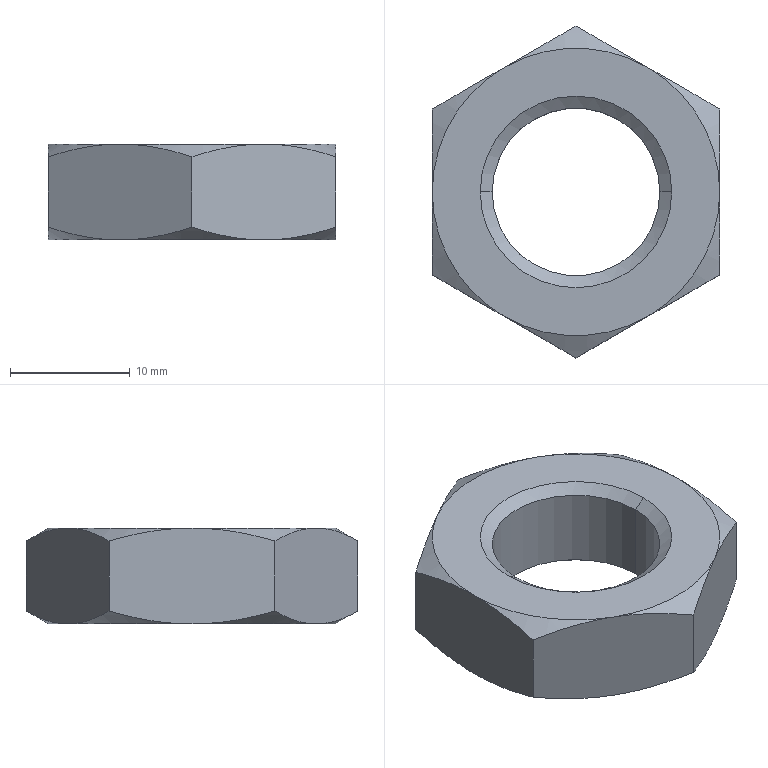Part | STEP file | hex thin nut chamfered gradeab_iso_ISO - 4035 - M16 - N | 1 solid | 28 faces | box 24 x 27.713 x 8 mm | volume 2696 mm3 | cone 16 | plane 8 | cylinder 4 | commonest cylinder face diameters 14 x2 16 x2
STEP:
#1=CARTESIAN_POINT('',(-8.,0.,-8.));
#2=VERTEX_POINT('',#1);
#3=CARTESIAN_POINT('',(8.,0.,-8.));
#4=VERTEX_POINT('',#3);
#5=CARTESIAN_POINT('',(0.,0.,-8.));
#6=DIRECTION('',(0.,0.,1.));
#7=DIRECTION('',(-1.,0.,0.));
#8=AXIS2_PLACEMENT_3D('',#5,#6,#7);
#9=CIRCLE('',#8,8.);
#10=EDGE_CURVE('',#2,#4,#9,.T.);
#11=ORIENTED_EDGE('',*,*,#10,.F.);
#12=CARTESIAN_POINT('',(-8.,0.,-7.975));
#13=VERTEX_POINT('',#12);
#14=CARTESIAN_POINT('',(-8.,0.,-25.038));
#15=DIRECTION('',(0.,0.,1.));
#16=VECTOR('',#15,1000.);
#17=LINE('',#14,#16);
#18=EDGE_CURVE('',#2,#13,#17,.T.);
#19=ORIENTED_EDGE('',*,*,#18,.T.);
#20=CARTESIAN_POINT('',(8.,0.,-7.975));
#21=VERTEX_POINT('',#20);
#22=CARTESIAN_POINT('',(0.,0.,-7.975));
#23=DIRECTION('',(0.,0.,1.));
#24=DIRECTION('',(1.,0.,0.));
#25=AXIS2_PLACEMENT_3D('',#22,#23,#24);
#26=CIRCLE('',#25,8.);
#27=EDGE_CURVE('',#13,#21,#26,.T.);
#28=ORIENTED_EDGE('',*,*,#27,.T.);
#29=CARTESIAN_POINT('',(8.,0.,-25.038));
#30=DIRECTION('',(0.,0.,1.));
#31=VECTOR('',#30,1000.);
#32=LINE('',#29,#31);
#33=EDGE_CURVE('',#4,#21,#32,.T.);
#34=ORIENTED_EDGE('',*,*,#33,.F.);
#35=EDGE_LOOP('',(#11,#19,#28,#34));
#36=FACE_OUTER_BOUND('',#35,.T.);
#37=CARTESIAN_POINT('',(0.,0.,-25.038));
#38=DIRECTION('',(0.,0.,1.));
#39=DIRECTION('',(1.,0.,0.));
#40=AXIS2_PLACEMENT_3D('',#37,#38,#39);
#41=CYLINDRICAL_SURFACE('',#40,8.);
#42=ADVANCED_FACE('',(#36),#41,.F.);
#43=CARTESIAN_POINT('',(-7.,0.,-7.274));
#44=VERTEX_POINT('',#43);
#45=CARTESIAN_POINT('',(7.,0.,-7.274));
#46=VERTEX_POINT('',#45);
#47=CARTESIAN_POINT('',(0.,0.,-7.274));
#48=DIRECTION('',(0.,0.,1.));
#49=DIRECTION('',(-1.,0.,0.));
#50=AXIS2_PLACEMENT_3D('',#47,#48,#49);
#51=CIRCLE('',#50,7.);
#52=EDGE_CURVE('',#44,#46,#51,.T.);
#53=ORIENTED_EDGE('',*,*,#52,.T.);
#54=CARTESIAN_POINT('',(8.,0.,-7.975));
#55=DIRECTION('',(0.8192,0.,-0.5736));
#56=VECTOR('',#55,1000.);
#57=LINE('',#54,#56);
#58=EDGE_CURVE('',#46,#21,#57,.T.);
#59=ORIENTED_EDGE('',*,*,#58,.T.);
#60=ORIENTED_EDGE('',*,*,#27,.F.);
#61=CARTESIAN_POINT('',(-8.,0.,-7.975));
#62=DIRECTION('',(-0.8192,0.,-0.5736));
#63=VECTOR('',#62,1000.);
#64=LINE('',#61,#63);
#65=EDGE_CURVE('',#44,#13,#64,.T.);
#66=ORIENTED_EDGE('',*,*,#65,.F.);
#67=EDGE_LOOP('',(#53,#59,#60,#66));
#68=FACE_OUTER_BOUND('',#67,.T.);
#69=CARTESIAN_POINT('',(0.,0.,-7.975));
#70=DIRECTION('',(0.,0.,-1.));
#71=DIRECTION('',(-1.,0.,0.));
#72=AXIS2_PLACEMENT_3D('',#69,#70,#71);
#73=CONICAL_SURFACE('',#72,8.,0.9599);
#74=ADVANCED_FACE('',(#68),#73,.F.);
#75=CARTESIAN_POINT('',(7.,0.,-0.7002));
#76=VERTEX_POINT('',#75);
#77=CARTESIAN_POINT('',(-7.,0.,-0.7002));
#78=VERTEX_POINT('',#77);
#79=CARTESIAN_POINT('',(0.,0.,-0.7002));
#80=DIRECTION('',(0.,0.,-1.));
#81=DIRECTION('',(1.,0.,0.));
#82=AXIS2_PLACEMENT_3D('',#79,#80,#81);
#83=CIRCLE('',#82,7.);
#84=EDGE_CURVE('',#76,#78,#83,.T.);
#85=ORIENTED_EDGE('',*,*,#84,.T.);
#86=CARTESIAN_POINT('',(-8.,0.,0.));
#87=VERTEX_POINT('',#86);
#88=CARTESIAN_POINT('',(-6.9,0.,-0.7702));
#89=DIRECTION('',(-0.8192,0.,0.5736));
#90=VECTOR('',#89,1000.);
#91=LINE('',#88,#90);
#92=EDGE_CURVE('',#78,#87,#91,.T.);
#93=ORIENTED_EDGE('',*,*,#92,.T.);
#94=CARTESIAN_POINT('',(8.,0.,0.));
#95=VERTEX_POINT('',#94);
#96=CARTESIAN_POINT('',(0.,0.,0.));
#97=DIRECTION('',(0.,0.,1.));
#98=DIRECTION('',(1.,0.,0.));
#99=AXIS2_PLACEMENT_3D('',#96,#97,#98);
#100=CIRCLE('',#99,8.);
#101=EDGE_CURVE('',#87,#95,#100,.T.);
#102=ORIENTED_EDGE('',*,*,#101,.T.);
#103=CARTESIAN_POINT('',(6.9,0.,-0.7702));
#104=DIRECTION('',(0.8192,0.,0.5736));
#105=VECTOR('',#104,1000.);
#106=LINE('',#103,#105);
#107=EDGE_CURVE('',#76,#95,#106,.T.);
#108=ORIENTED_EDGE('',*,*,#107,.F.);
#109=EDGE_LOOP('',(#85,#93,#102,#108));
#110=FACE_OUTER_BOUND('',#109,.T.);
#111=CARTESIAN_POINT('',(0.,0.,-0.7702));
#112=DIRECTION('',(0.,0.,1.));
#113=DIRECTION('',(1.,0.,0.));
#114=AXIS2_PLACEMENT_3D('',#111,#112,#113);
#115=CONICAL_SURFACE('',#114,6.9,0.9599);
#116=ADVANCED_FACE('',(#110),#115,.F.);
#117=ORIENTED_EDGE('',*,*,#52,.F.);
#118=CARTESIAN_POINT('',(-7.,0.,-8.));
#119=DIRECTION('',(0.,0.,1.));
#120=VECTOR('',#119,1000.);
#121=LINE('',#118,#120);
#122=EDGE_CURVE('',#44,#78,#121,.T.);
#123=ORIENTED_EDGE('',*,*,#122,.T.);
#124=ORIENTED_EDGE('',*,*,#84,.F.);
#125=CARTESIAN_POINT('',(7.,0.,-8.));
#126=DIRECTION('',(0.,0.,1.));
#127=VECTOR('',#126,1000.);
#128=LINE('',#125,#127);
#129=EDGE_CURVE('',#46,#76,#128,.T.);
#130=ORIENTED_EDGE('',*,*,#129,.F.);
#131=EDGE_LOOP('',(#117,#123,#124,#130));
#132=FACE_OUTER_BOUND('',#131,.T.);
#133=CARTESIAN_POINT('',(0.,0.,-8.));
#134=DIRECTION('',(0.,0.,1.));
#135=DIRECTION('',(1.,0.,0.));
#136=AXIS2_PLACEMENT_3D('',#133,#134,#135);
#137=CYLINDRICAL_SURFACE('',#136,7.);
#138=ADVANCED_FACE('',(#132),#137,.F.);
#139=ORIENTED_EDGE('',*,*,#122,.F.);
#140=CARTESIAN_POINT('',(0.,0.,-7.274));
#141=DIRECTION('',(0.,0.,1.));
#142=DIRECTION('',(-1.,0.,0.));
#143=AXIS2_PLACEMENT_3D('',#140,#141,#142);
#144=CIRCLE('',#143,7.);
#145=EDGE_CURVE('',#46,#44,#144,.T.);
#146=ORIENTED_EDGE('',*,*,#145,.F.);
#147=ORIENTED_EDGE('',*,*,#129,.T.);
#148=CARTESIAN_POINT('',(0.,0.,-0.7002));
#149=DIRECTION('',(0.,0.,-1.));
#150=DIRECTION('',(1.,0.,0.));
#151=AXIS2_PLACEMENT_3D('',#148,#149,#150);
#152=CIRCLE('',#151,7.);
#153=EDGE_CURVE('',#78,#76,#152,.T.);
#154=ORIENTED_EDGE('',*,*,#153,.F.);
#155=EDGE_LOOP('',(#139,#146,#147,#154));
#156=FACE_OUTER_BOUND('',#155,.T.);
#157=CARTESIAN_POINT('',(0.,0.,-8.));
#158=DIRECTION('',(0.,0.,1.));
#159=DIRECTION('',(1.,0.,0.));
#160=AXIS2_PLACEMENT_3D('',#157,#158,#159);
#161=CYLINDRICAL_SURFACE('',#160,7.);
#162=ADVANCED_FACE('',(#156),#161,.F.);
#163=CARTESIAN_POINT('',(-12.,6.928,-6.928));
#164=VERTEX_POINT('',#163);
#165=CARTESIAN_POINT('',(-12.,6.928,-1.072));
#166=VERTEX_POINT('',#165);
#167=CARTESIAN_POINT('',(-12.,6.928,-8.));
#168=DIRECTION('',(0.,0.,1.));
#169=VECTOR('',#168,1000.);
#170=LINE('',#167,#169);
#171=EDGE_CURVE('',#164,#166,#170,.T.);
#172=ORIENTED_EDGE('',*,*,#171,.T.);
#173=CARTESIAN_POINT('',(-6.,10.392,0.));
#174=VERTEX_POINT('',#173);
#175=CARTESIAN_POINT('',(-12.,6.928,-1.072));
#176=CARTESIAN_POINT('',(-11.018,7.495,-0.7446));
#177=CARTESIAN_POINT('',(-10.03,8.066,-0.4751));
#178=CARTESIAN_POINT('',(-8.032,9.219,-0.1021));
#179=CARTESIAN_POINT('',(-7.022,9.802,0.));
#180=CARTESIAN_POINT('',(-6.,10.392,0.));
#181=B_SPLINE_CURVE_WITH_KNOTS('',3,(#175,#176,#177,#178,#179,#180),.UNSPECIFIED.,.F.,.F.,(4,2,4),(0.000000238,0.003505,0.00701),.UNSPECIFIED.);
#182=EDGE_CURVE('',#166,#174,#181,.T.);
#183=ORIENTED_EDGE('',*,*,#182,.T.);
#184=CARTESIAN_POINT('',(0.,13.856,-1.072));
#185=VERTEX_POINT('',#184);
#186=CARTESIAN_POINT('',(-6.,10.392,0.));
#187=CARTESIAN_POINT('',(-5.491,10.686,0.));
#188=CARTESIAN_POINT('',(-4.979,10.982,-0.02533));
#189=CARTESIAN_POINT('',(-3.967,11.566,-0.1234));
#190=CARTESIAN_POINT('',(-3.465,11.856,-0.196));
#191=CARTESIAN_POINT('',(-1.966,12.721,-0.476));
#192=CARTESIAN_POINT('',(-0.9791,13.291,-0.7454));
#193=CARTESIAN_POINT('',(0.,13.856,-1.072));
#194=B_SPLINE_CURVE_WITH_KNOTS('',3,(#186,#187,#188,#189,#190,#191,#192,#193),.UNSPECIFIED.,.F.,.F.,(4,2,2,4),(0.00701,0.008756,0.0105,0.01399),.UNSPECIFIED.);
#195=EDGE_CURVE('',#174,#185,#194,.T.);
#196=ORIENTED_EDGE('',*,*,#195,.T.);
#197=CARTESIAN_POINT('',(0.,13.856,-6.928));
#198=VERTEX_POINT('',#197);
#199=CARTESIAN_POINT('',(0.,13.856,-8.));
#200=DIRECTION('',(0.,0.,1.));
#201=VECTOR('',#200,1000.);
#202=LINE('',#199,#201);
#203=EDGE_CURVE('',#198,#185,#202,.T.);
#204=ORIENTED_EDGE('',*,*,#203,.F.);
#205=CARTESIAN_POINT('',(-6.,10.392,-8.));
#206=VERTEX_POINT('',#205);
#207=CARTESIAN_POINT('',(-6.,10.392,-8.));
#208=CARTESIAN_POINT('',(-5.491,10.686,-8.));
#209=CARTESIAN_POINT('',(-4.979,10.982,-7.975));
#210=CARTESIAN_POINT('',(-3.967,11.566,-7.877));
#211=CARTESIAN_POINT('',(-3.465,11.856,-7.804));
#212=CARTESIAN_POINT('',(-1.966,12.721,-7.524));
#213=CARTESIAN_POINT('',(-0.9791,13.291,-7.255));
#214=CARTESIAN_POINT('',(0.,13.856,-6.928));
#215=B_SPLINE_CURVE_WITH_KNOTS('',3,(#207,#208,#209,#210,#211,#212,#213,#214),.UNSPECIFIED.,.F.,.F.,(4,2,2,4),(0.00701,0.008756,0.0105,0.01399),.UNSPECIFIED.);
#216=EDGE_CURVE('',#206,#198,#215,.T.);
#217=ORIENTED_EDGE('',*,*,#216,.F.);
#218=CARTESIAN_POINT('',(-12.,6.928,-6.928));
#219=CARTESIAN_POINT('',(-11.018,7.495,-7.255));
#220=CARTESIAN_POINT('',(-10.03,8.066,-7.525));
#221=CARTESIAN_POINT('',(-8.032,9.219,-7.898));
#222=CARTESIAN_POINT('',(-7.022,9.802,-8.));
#223=CARTESIAN_POINT('',(-6.,10.392,-8.));
#224=B_SPLINE_CURVE_WITH_KNOTS('',3,(#218,#219,#220,#221,#222,#223),.UNSPECIFIED.,.F.,.F.,(4,2,4),(0.000000238,0.003505,0.00701),.UNSPECIFIED.);
#225=EDGE_CURVE('',#164,#206,#224,.T.);
#226=ORIENTED_EDGE('',*,*,#225,.F.);
#227=EDGE_LOOP('',(#172,#183,#196,#204,#217,#226));
#228=FACE_OUTER_BOUND('',#227,.T.);
#229=CARTESIAN_POINT('',(0.,13.856,-8.));
#230=DIRECTION('',(-0.5,0.866,0.));
#231=DIRECTION('',(-0.866,-0.5,0.));
#232=AXIS2_PLACEMENT_3D('',#229,#230,#231);
#233=PLANE('',#232);
#234=ADVANCED_FACE('',(#228),#233,.T.);
#235=ORIENTED_EDGE('',*,*,#203,.T.);
#236=CARTESIAN_POINT('',(6.,10.392,0.));
#237=VERTEX_POINT('',#236);
#238=CARTESIAN_POINT('',(0.,13.856,-1.072));
#239=CARTESIAN_POINT('',(0.9815,13.29,-0.7446));
#240=CARTESIAN_POINT('',(1.97,12.719,-0.4751));
#241=CARTESIAN_POINT('',(3.968,11.565,-0.1021));
#242=CARTESIAN_POINT('',(4.978,10.982,0.));
#243=CARTESIAN_POINT('',(6.,10.392,0.));
#244=B_SPLINE_CURVE_WITH_KNOTS('',3,(#238,#239,#240,#241,#242,#243),.UNSPECIFIED.,.F.,.F.,(4,2,4),(0.000000238,0.003505,0.00701),.UNSPECIFIED.);
#245=EDGE_CURVE('',#185,#237,#244,.T.);
#246=ORIENTED_EDGE('',*,*,#245,.T.);
#247=CARTESIAN_POINT('',(12.,6.928,-1.072));
#248=VERTEX_POINT('',#247);
#249=CARTESIAN_POINT('',(6.,10.392,0.));
#250=CARTESIAN_POINT('',(6.509,10.098,0.));
#251=CARTESIAN_POINT('',(7.021,9.803,-0.02533));
#252=CARTESIAN_POINT('',(8.033,9.219,-0.1234));
#253=CARTESIAN_POINT('',(8.535,8.929,-0.196));
#254=CARTESIAN_POINT('',(10.034,8.063,-0.476));
#255=CARTESIAN_POINT('',(11.021,7.493,-0.7454));
#256=CARTESIAN_POINT('',(12.,6.928,-1.072));
#257=B_SPLINE_CURVE_WITH_KNOTS('',3,(#249,#250,#251,#252,#253,#254,#255,#256),.UNSPECIFIED.,.F.,.F.,(4,2,2,4),(0.00701,0.008756,0.0105,0.01399),.UNSPECIFIED.);
#258=EDGE_CURVE('',#237,#248,#257,.T.);
#259=ORIENTED_EDGE('',*,*,#258,.T.);
#260=CARTESIAN_POINT('',(12.,6.928,-6.928));
#261=VERTEX_POINT('',#260);
#262=CARTESIAN_POINT('',(12.,6.928,-8.));
#263=DIRECTION('',(0.,0.,1.));
#264=VECTOR('',#263,1000.);
#265=LINE('',#262,#264);
#266=EDGE_CURVE('',#261,#248,#265,.T.);
#267=ORIENTED_EDGE('',*,*,#266,.F.);
#268=CARTESIAN_POINT('',(6.,10.392,-8.));
#269=VERTEX_POINT('',#268);
#270=CARTESIAN_POINT('',(6.,10.392,-8.));
#271=CARTESIAN_POINT('',(6.509,10.098,-8.));
#272=CARTESIAN_POINT('',(7.021,9.803,-7.975));
#273=CARTESIAN_POINT('',(8.033,9.219,-7.877));
#274=CARTESIAN_POINT('',(8.535,8.929,-7.804));
#275=CARTESIAN_POINT('',(10.034,8.063,-7.524));
#276=CARTESIAN_POINT('',(11.021,7.493,-7.255));
#277=CARTESIAN_POINT('',(12.,6.928,-6.928));
#278=B_SPLINE_CURVE_WITH_KNOTS('',3,(#270,#271,#272,#273,#274,#275,#276,#277),.UNSPECIFIED.,.F.,.F.,(4,2,2,4),(0.00701,0.008756,0.0105,0.01399),.UNSPECIFIED.);
#279=EDGE_CURVE('',#269,#261,#278,.T.);
#280=ORIENTED_EDGE('',*,*,#279,.F.);
#281=CARTESIAN_POINT('',(0.,13.856,-6.928));
#282=CARTESIAN_POINT('',(0.9815,13.29,-7.255));
#283=CARTESIAN_POINT('',(1.97,12.719,-7.525));
#284=CARTESIAN_POINT('',(3.968,11.565,-7.898));
#285=CARTESIAN_POINT('',(4.978,10.982,-8.));
#286=CARTESIAN_POINT('',(6.,10.392,-8.));
#287=B_SPLINE_CURVE_WITH_KNOTS('',3,(#281,#282,#283,#284,#285,#286),.UNSPECIFIED.,.F.,.F.,(4,2,4),(0.000000238,0.003505,0.00701),.UNSPECIFIED.);
#288=EDGE_CURVE('',#198,#269,#287,.T.);
#289=ORIENTED_EDGE('',*,*,#288,.F.);
#290=EDGE_LOOP('',(#235,#246,#259,#267,#280,#289));
#291=FACE_OUTER_BOUND('',#290,.T.);
#292=CARTESIAN_POINT('',(12.,6.928,-8.));
#293=DIRECTION('',(0.5,0.866,0.));
#294=DIRECTION('',(-0.866,0.5,0.));
#295=AXIS2_PLACEMENT_3D('',#292,#293,#294);
#296=PLANE('',#295);
#297=ADVANCED_FACE('',(#291),#296,.T.);
#298=CARTESIAN_POINT('',(12.,-6.928,-1.072));
#299=VERTEX_POINT('',#298);
#300=CARTESIAN_POINT('',(12.,0.,0.));
#301=VERTEX_POINT('',#300);
#302=CARTESIAN_POINT('',(12.,-6.928,-1.072));
#303=CARTESIAN_POINT('',(12.,-5.801,-0.7465));
#304=CARTESIAN_POINT('',(12.,-4.647,-0.4737));
#305=CARTESIAN_POINT('',(12.,-2.334,-0.1006));
#306=CARTESIAN_POINT('',(12.,-1.171,0.));
#307=CARTESIAN_POINT('',(12.,0.,0.));
#308=B_SPLINE_CURVE_WITH_KNOTS('',3,(#302,#303,#304,#305,#306,#307),.UNSPECIFIED.,.F.,.F.,(4,2,4),(0.01236,0.01587,0.01937),.UNSPECIFIED.);
#309=EDGE_CURVE('',#299,#301,#308,.T.);
#310=ORIENTED_EDGE('',*,*,#309,.F.);
#311=CARTESIAN_POINT('',(12.,-6.928,-6.928));
#312=VERTEX_POINT('',#311);
#313=CARTESIAN_POINT('',(12.,-6.928,-8.));
#314=DIRECTION('',(0.,0.,1.));
#315=VECTOR('',#314,1000.);
#316=LINE('',#313,#315);
#317=EDGE_CURVE('',#312,#299,#316,.T.);
#318=ORIENTED_EDGE('',*,*,#317,.F.);
#319=CARTESIAN_POINT('',(12.,0.,-8.));
#320=VERTEX_POINT('',#319);
#321=CARTESIAN_POINT('',(12.,-6.928,-6.928));
#322=CARTESIAN_POINT('',(12.,-5.801,-7.253));
#323=CARTESIAN_POINT('',(12.,-4.647,-7.526));
#324=CARTESIAN_POINT('',(12.,-2.334,-7.899));
#325=CARTESIAN_POINT('',(12.,-1.171,-8.));
#326=CARTESIAN_POINT('',(12.,0.,-8.));
#327=B_SPLINE_CURVE_WITH_KNOTS('',3,(#321,#322,#323,#324,#325,#326),.UNSPECIFIED.,.F.,.F.,(4,2,4),(0.01236,0.01587,0.01937),.UNSPECIFIED.);
#328=EDGE_CURVE('',#312,#320,#327,.T.);
#329=ORIENTED_EDGE('',*,*,#328,.T.);
#330=CARTESIAN_POINT('',(12.,0.,-8.));
#331=CARTESIAN_POINT('',(12.,0.5857,-8.));
#332=CARTESIAN_POINT('',(12.,1.173,-7.975));
#333=CARTESIAN_POINT('',(12.,2.352,-7.876));
#334=CARTESIAN_POINT('',(12.,2.937,-7.803));
#335=CARTESIAN_POINT('',(12.,4.673,-7.521));
#336=CARTESIAN_POINT('',(12.,5.808,-7.252));
#337=CARTESIAN_POINT('',(12.,6.928,-6.928));
#338=B_SPLINE_CURVE_WITH_KNOTS('',3,(#330,#331,#332,#333,#334,#335,#336,#337),.UNSPECIFIED.,.F.,.F.,(4,2,2,4),(0.01937,0.02112,0.02288,0.02638),.UNSPECIFIED.);
#339=EDGE_CURVE('',#320,#261,#338,.T.);
#340=ORIENTED_EDGE('',*,*,#339,.T.);
#341=ORIENTED_EDGE('',*,*,#266,.T.);
#342=CARTESIAN_POINT('',(12.,0.,0.));
#343=CARTESIAN_POINT('',(12.,0.5857,0.));
#344=CARTESIAN_POINT('',(12.,1.173,-0.02489));
#345=CARTESIAN_POINT('',(12.,2.352,-0.1238));
#346=CARTESIAN_POINT('',(12.,2.937,-0.1973));
#347=CARTESIAN_POINT('',(12.,4.673,-0.4791));
#348=CARTESIAN_POINT('',(12.,5.808,-0.7484));
#349=CARTESIAN_POINT('',(12.,6.928,-1.072));
#350=B_SPLINE_CURVE_WITH_KNOTS('',3,(#342,#343,#344,#345,#346,#347,#348,#349),.UNSPECIFIED.,.F.,.F.,(4,2,2,4),(0.01937,0.02112,0.02288,0.02638),.UNSPECIFIED.);
#351=EDGE_CURVE('',#301,#248,#350,.T.);
#352=ORIENTED_EDGE('',*,*,#351,.F.);
#353=EDGE_LOOP('',(#310,#318,#329,#340,#341,#352));
#354=FACE_OUTER_BOUND('',#353,.T.);
#355=CARTESIAN_POINT('',(12.,6.928,-8.));
#356=DIRECTION('',(-1.,0.,0.));
#357=DIRECTION('',(0.,0.,1.));
#358=AXIS2_PLACEMENT_3D('',#355,#356,#357);
#359=PLANE('',#358);
#360=ADVANCED_FACE('',(#354),#359,.F.);
#361=ORIENTED_EDGE('',*,*,#317,.T.);
#362=CARTESIAN_POINT('',(6.,-10.392,0.));
#363=VERTEX_POINT('',#362);
#364=CARTESIAN_POINT('',(12.,-6.928,-1.072));
#365=CARTESIAN_POINT('',(11.018,-7.495,-0.7446));
#366=CARTESIAN_POINT('',(10.03,-8.066,-0.4751));
#367=CARTESIAN_POINT('',(8.032,-9.219,-0.1021));
#368=CARTESIAN_POINT('',(7.022,-9.802,0.));
#369=CARTESIAN_POINT('',(6.,-10.392,0.));
#370=B_SPLINE_CURVE_WITH_KNOTS('',3,(#364,#365,#366,#367,#368,#369),.UNSPECIFIED.,.F.,.F.,(4,2,4),(0.000000238,0.003505,0.00701),.UNSPECIFIED.);
#371=EDGE_CURVE('',#299,#363,#370,.T.);
#372=ORIENTED_EDGE('',*,*,#371,.T.);
#373=CARTESIAN_POINT('',(0.,-13.856,-1.072));
#374=VERTEX_POINT('',#373);
#375=CARTESIAN_POINT('',(6.,-10.392,0.));
#376=CARTESIAN_POINT('',(5.491,-10.686,0.));
#377=CARTESIAN_POINT('',(4.979,-10.982,-0.02533));
#378=CARTESIAN_POINT('',(3.967,-11.566,-0.1234));
#379=CARTESIAN_POINT('',(3.465,-11.856,-0.196));
#380=CARTESIAN_POINT('',(1.966,-12.721,-0.476));
#381=CARTESIAN_POINT('',(0.9791,-13.291,-0.7454));
#382=CARTESIAN_POINT('',(0.,-13.856,-1.072));
#383=B_SPLINE_CURVE_WITH_KNOTS('',3,(#375,#376,#377,#378,#379,#380,#381,#382),.UNSPECIFIED.,.F.,.F.,(4,2,2,4),(0.00701,0.008756,0.0105,0.01399),.UNSPECIFIED.);
#384=EDGE_CURVE('',#363,#374,#383,.T.);
#385=ORIENTED_EDGE('',*,*,#384,.T.);
#386=CARTESIAN_POINT('',(0.,-13.856,-6.928));
#387=VERTEX_POINT('',#386);
#388=CARTESIAN_POINT('',(0.,-13.856,-8.));
#389=DIRECTION('',(0.,0.,1.));
#390=VECTOR('',#389,1000.);
#391=LINE('',#388,#390);
#392=EDGE_CURVE('',#387,#374,#391,.T.);
#393=ORIENTED_EDGE('',*,*,#392,.F.);
#394=CARTESIAN_POINT('',(6.,-10.392,-8.));
#395=VERTEX_POINT('',#394);
#396=CARTESIAN_POINT('',(6.,-10.392,-8.));
#397=CARTESIAN_POINT('',(5.491,-10.686,-8.));
#398=CARTESIAN_POINT('',(4.979,-10.982,-7.975));
#399=CARTESIAN_POINT('',(3.967,-11.566,-7.877));
#400=CARTESIAN_POINT('',(3.465,-11.856,-7.804));
#401=CARTESIAN_POINT('',(1.966,-12.721,-7.524));
#402=CARTESIAN_POINT('',(0.9791,-13.291,-7.255));
#403=CARTESIAN_POINT('',(0.,-13.856,-6.928));
#404=B_SPLINE_CURVE_WITH_KNOTS('',3,(#396,#397,#398,#399,#400,#401,#402,#403),.UNSPECIFIED.,.F.,.F.,(4,2,2,4),(0.00701,0.008756,0.0105,0.01399),.UNSPECIFIED.);
#405=EDGE_CURVE('',#395,#387,#404,.T.);
#406=ORIENTED_EDGE('',*,*,#405,.F.);
#407=CARTESIAN_POINT('',(12.,-6.928,-6.928));
#408=CARTESIAN_POINT('',(11.018,-7.495,-7.255));
#409=CARTESIAN_POINT('',(10.03,-8.066,-7.525));
#410=CARTESIAN_POINT('',(8.032,-9.219,-7.898));
#411=CARTESIAN_POINT('',(7.022,-9.802,-8.));
#412=CARTESIAN_POINT('',(6.,-10.392,-8.));
#413=B_SPLINE_CURVE_WITH_KNOTS('',3,(#407,#408,#409,#410,#411,#412),.UNSPECIFIED.,.F.,.F.,(4,2,4),(0.000000238,0.003505,0.00701),.UNSPECIFIED.);
#414=EDGE_CURVE('',#312,#395,#413,.T.);
#415=ORIENTED_EDGE('',*,*,#414,.F.);
#416=EDGE_LOOP('',(#361,#372,#385,#393,#406,#415));
#417=FACE_OUTER_BOUND('',#416,.T.);
#418=CARTESIAN_POINT('',(0.,-13.856,-8.));
#419=DIRECTION('',(0.5,-0.866,0.));
#420=DIRECTION('',(0.866,0.5,0.));
#421=AXIS2_PLACEMENT_3D('',#418,#419,#420);
#422=PLANE('',#421);
#423=ADVANCED_FACE('',(#417),#422,.T.);
#424=ORIENTED_EDGE('',*,*,#392,.T.);
#425=CARTESIAN_POINT('',(-6.,-10.392,0.));
#426=VERTEX_POINT('',#425);
#427=CARTESIAN_POINT('',(0.,-13.856,-1.072));
#428=CARTESIAN_POINT('',(-0.9815,-13.29,-0.7446));
#429=CARTESIAN_POINT('',(-1.97,-12.719,-0.4751));
#430=CARTESIAN_POINT('',(-3.968,-11.565,-0.1021));
#431=CARTESIAN_POINT('',(-4.978,-10.982,0.));
#432=CARTESIAN_POINT('',(-6.,-10.392,0.));
#433=B_SPLINE_CURVE_WITH_KNOTS('',3,(#427,#428,#429,#430,#431,#432),.UNSPECIFIED.,.F.,.F.,(4,2,4),(0.000000238,0.003505,0.00701),.UNSPECIFIED.);
#434=EDGE_CURVE('',#374,#426,#433,.T.);
#435=ORIENTED_EDGE('',*,*,#434,.T.);
#436=CARTESIAN_POINT('',(-12.,-6.928,-1.072));
#437=VERTEX_POINT('',#436);
#438=CARTESIAN_POINT('',(-6.,-10.392,0.));
#439=CARTESIAN_POINT('',(-6.509,-10.098,0.));
#440=CARTESIAN_POINT('',(-7.021,-9.803,-0.02533));
#441=CARTESIAN_POINT('',(-8.033,-9.219,-0.1234));
#442=CARTESIAN_POINT('',(-8.535,-8.929,-0.196));
#443=CARTESIAN_POINT('',(-10.034,-8.063,-0.476));
#444=CARTESIAN_POINT('',(-11.021,-7.493,-0.7454));
#445=CARTESIAN_POINT('',(-12.,-6.928,-1.072));
#446=B_SPLINE_CURVE_WITH_KNOTS('',3,(#438,#439,#440,#441,#442,#443,#444,#445),.UNSPECIFIED.,.F.,.F.,(4,2,2,4),(0.00701,0.008756,0.0105,0.01399),.UNSPECIFIED.);
#447=EDGE_CURVE('',#426,#437,#446,.T.);
#448=ORIENTED_EDGE('',*,*,#447,.T.);
#449=CARTESIAN_POINT('',(-12.,-6.928,-6.928));
#450=VERTEX_POINT('',#449);
#451=CARTESIAN_POINT('',(-12.,-6.928,-8.));
#452=DIRECTION('',(0.,0.,1.));
#453=VECTOR('',#452,1000.);
#454=LINE('',#451,#453);
#455=EDGE_CURVE('',#450,#437,#454,.T.);
#456=ORIENTED_EDGE('',*,*,#455,.F.);
#457=CARTESIAN_POINT('',(-6.,-10.392,-8.));
#458=VERTEX_POINT('',#457);
#459=CARTESIAN_POINT('',(-6.,-10.392,-8.));
#460=CARTESIAN_POINT('',(-6.509,-10.098,-8.));
#461=CARTESIAN_POINT('',(-7.021,-9.803,-7.975));
#462=CARTESIAN_POINT('',(-8.033,-9.219,-7.877));
#463=CARTESIAN_POINT('',(-8.535,-8.929,-7.804));
#464=CARTESIAN_POINT('',(-10.034,-8.063,-7.524));
#465=CARTESIAN_POINT('',(-11.021,-7.493,-7.255));
#466=CARTESIAN_POINT('',(-12.,-6.928,-6.928));
#467=B_SPLINE_CURVE_WITH_KNOTS('',3,(#459,#460,#461,#462,#463,#464,#465,#466),.UNSPECIFIED.,.F.,.F.,(4,2,2,4),(0.00701,0.008756,0.0105,0.01399),.UNSPECIFIED.);
#468=EDGE_CURVE('',#458,#450,#467,.T.);
#469=ORIENTED_EDGE('',*,*,#468,.F.);
#470=CARTESIAN_POINT('',(0.,-13.856,-6.928));
#471=CARTESIAN_POINT('',(-0.9815,-13.29,-7.255));
#472=CARTESIAN_POINT('',(-1.97,-12.719,-7.525));
#473=CARTESIAN_POINT('',(-3.968,-11.565,-7.898));
#474=CARTESIAN_POINT('',(-4.978,-10.982,-8.));
#475=CARTESIAN_POINT('',(-6.,-10.392,-8.));
#476=B_SPLINE_CURVE_WITH_KNOTS('',3,(#470,#471,#472,#473,#474,#475),.UNSPECIFIED.,.F.,.F.,(4,2,4),(0.000000238,0.003505,0.00701),.UNSPECIFIED.);
#477=EDGE_CURVE('',#387,#458,#476,.T.);
#478=ORIENTED_EDGE('',*,*,#477,.F.);
#479=EDGE_LOOP('',(#424,#435,#448,#456,#469,#478));
#480=FACE_OUTER_BOUND('',#479,.T.);
#481=CARTESIAN_POINT('',(-12.,-6.928,-8.));
#482=DIRECTION('',(-0.5,-0.866,0.));
#483=DIRECTION('',(0.866,-0.5,0.));
#484=AXIS2_PLACEMENT_3D('',#481,#482,#483);
#485=PLANE('',#484);
#486=ADVANCED_FACE('',(#480),#485,.T.);
#487=ORIENTED_EDGE('',*,*,#455,.T.);
#488=CARTESIAN_POINT('',(-12.,0.,0.));
#489=VERTEX_POINT('',#488);
#490=CARTESIAN_POINT('',(-12.,-6.928,-1.072));
#491=CARTESIAN_POINT('',(-12.,-5.801,-0.7465));
#492=CARTESIAN_POINT('',(-12.,-4.647,-0.4737));
#493=CARTESIAN_POINT('',(-12.,-2.334,-0.1006));
#494=CARTESIAN_POINT('',(-12.,-1.171,0.));
#495=CARTESIAN_POINT('',(-12.,0.,0.));
#496=B_SPLINE_CURVE_WITH_KNOTS('',3,(#490,#491,#492,#493,#494,#495),.UNSPECIFIED.,.F.,.F.,(4,2,4),(0.01236,0.01587,0.01937),.UNSPECIFIED.);
#497=EDGE_CURVE('',#437,#489,#496,.T.);
#498=ORIENTED_EDGE('',*,*,#497,.T.);
#499=CARTESIAN_POINT('',(-12.,0.,0.));
#500=CARTESIAN_POINT('',(-12.,0.5857,0.));
#501=CARTESIAN_POINT('',(-12.,1.173,-0.02489));
#502=CARTESIAN_POINT('',(-12.,2.352,-0.1238));
#503=CARTESIAN_POINT('',(-12.,2.937,-0.1973));
#504=CARTESIAN_POINT('',(-12.,4.673,-0.4791));
#505=CARTESIAN_POINT('',(-12.,5.808,-0.7484));
#506=CARTESIAN_POINT('',(-12.,6.928,-1.072));
#507=B_SPLINE_CURVE_WITH_KNOTS('',3,(#499,#500,#501,#502,#503,#504,#505,#506),.UNSPECIFIED.,.F.,.F.,(4,2,2,4),(0.01937,0.02112,0.02288,0.02638),.UNSPECIFIED.);
#508=EDGE_CURVE('',#489,#166,#507,.T.);
#509=ORIENTED_EDGE('',*,*,#508,.T.);
#510=ORIENTED_EDGE('',*,*,#171,.F.);
#511=CARTESIAN_POINT('',(-12.,0.,-8.));
#512=VERTEX_POINT('',#511);
#513=CARTESIAN_POINT('',(-12.,0.,-8.));
#514=CARTESIAN_POINT('',(-12.,0.5857,-8.));
#515=CARTESIAN_POINT('',(-12.,1.173,-7.975));
#516=CARTESIAN_POINT('',(-12.,2.352,-7.876));
#517=CARTESIAN_POINT('',(-12.,2.937,-7.803));
#518=CARTESIAN_POINT('',(-12.,4.673,-7.521));
#519=CARTESIAN_POINT('',(-12.,5.808,-7.252));
#520=CARTESIAN_POINT('',(-12.,6.928,-6.928));
#521=B_SPLINE_CURVE_WITH_KNOTS('',3,(#513,#514,#515,#516,#517,#518,#519,#520),.UNSPECIFIED.,.F.,.F.,(4,2,2,4),(0.01937,0.02112,0.02288,0.02638),.UNSPECIFIED.);
#522=EDGE_CURVE('',#512,#164,#521,.T.);
#523=ORIENTED_EDGE('',*,*,#522,.F.);
#524=CARTESIAN_POINT('',(-12.,-6.928,-6.928));
#525=CARTESIAN_POINT('',(-12.,-5.801,-7.253));
#526=CARTESIAN_POINT('',(-12.,-4.647,-7.526));
#527=CARTESIAN_POINT('',(-12.,-2.334,-7.899));
#528=CARTESIAN_POINT('',(-12.,-1.171,-8.));
#529=CARTESIAN_POINT('',(-12.,0.,-8.));
#530=B_SPLINE_CURVE_WITH_KNOTS('',3,(#524,#525,#526,#527,#528,#529),.UNSPECIFIED.,.F.,.F.,(4,2,4),(0.01236,0.01587,0.01937),.UNSPECIFIED.);
#531=EDGE_CURVE('',#450,#512,#530,.T.);
#532=ORIENTED_EDGE('',*,*,#531,.F.);
#533=EDGE_LOOP('',(#487,#498,#509,#510,#523,#532));
#534=FACE_OUTER_BOUND('',#533,.T.);
#535=CARTESIAN_POINT('',(-12.,6.928,-8.));
#536=DIRECTION('',(-1.,0.,0.));
#537=DIRECTION('',(0.,0.,1.));
#538=AXIS2_PLACEMENT_3D('',#535,#536,#537);
#539=PLANE('',#538);
#540=ADVANCED_FACE('',(#534),#539,.T.);
#541=CARTESIAN_POINT('',(0.,0.,0.));
#542=DIRECTION('',(0.,0.,1.));
#543=DIRECTION('',(1.,0.,0.));
#544=AXIS2_PLACEMENT_3D('',#541,#542,#543);
#545=CIRCLE('',#544,8.);
#546=EDGE_CURVE('',#95,#87,#545,.T.);
#547=ORIENTED_EDGE('',*,*,#546,.F.);
#548=ORIENTED_EDGE('',*,*,#101,.F.);
#549=EDGE_LOOP('',(#547,#548));
#550=FACE_BOUND('',#549,.T.);
#551=CARTESIAN_POINT('',(0.,0.,0.));
#552=DIRECTION('',(0.,0.,-1.));
#553=DIRECTION('',(-1.,0.,0.));
#554=AXIS2_PLACEMENT_3D('',#551,#552,#553);
#555=CIRCLE('',#554,12.);
#556=EDGE_CURVE('',#489,#174,#555,.T.);
#557=ORIENTED_EDGE('',*,*,#556,.F.);
#558=CARTESIAN_POINT('',(0.,0.,0.));
#559=DIRECTION('',(0.,0.,-1.));
#560=DIRECTION('',(-1.,0.,0.));
#561=AXIS2_PLACEMENT_3D('',#558,#559,#560);
#562=CIRCLE('',#561,12.);
#563=EDGE_CURVE('',#426,#489,#562,.T.);
#564=ORIENTED_EDGE('',*,*,#563,.F.);
#565=CARTESIAN_POINT('',(0.,0.,0.));
#566=DIRECTION('',(0.,0.,-1.));
#567=DIRECTION('',(-1.,0.,0.));
#568=AXIS2_PLACEMENT_3D('',#565,#566,#567);
#569=CIRCLE('',#568,12.);
#570=EDGE_CURVE('',#363,#426,#569,.T.);
#571=ORIENTED_EDGE('',*,*,#570,.F.);
#572=CARTESIAN_POINT('',(0.,0.,0.));
#573=DIRECTION('',(0.,0.,-1.));
#574=DIRECTION('',(-1.,0.,0.));
#575=AXIS2_PLACEMENT_3D('',#572,#573,#574);
#576=CIRCLE('',#575,12.);
#577=EDGE_CURVE('',#301,#363,#576,.T.);
#578=ORIENTED_EDGE('',*,*,#577,.F.);
#579=CARTESIAN_POINT('',(0.,0.,0.));
#580=DIRECTION('',(0.,0.,1.));
#581=DIRECTION('',(1.,0.,0.));
#582=AXIS2_PLACEMENT_3D('',#579,#580,#581);
#583=CIRCLE('',#582,12.);
#584=EDGE_CURVE('',#301,#237,#583,.T.);
#585=ORIENTED_EDGE('',*,*,#584,.T.);
#586=CARTESIAN_POINT('',(0.,0.,0.));
#587=DIRECTION('',(0.,0.,-1.));
#588=DIRECTION('',(-1.,0.,0.));
#589=AXIS2_PLACEMENT_3D('',#586,#587,#588);
#590=CIRCLE('',#589,12.);
#591=EDGE_CURVE('',#174,#237,#590,.T.);
#592=ORIENTED_EDGE('',*,*,#591,.F.);
#593=EDGE_LOOP('',(#557,#564,#571,#578,#585,#592));
#594=FACE_OUTER_BOUND('',#593,.T.);
#595=CARTESIAN_POINT('',(0.,13.856,0.));
#596=DIRECTION('',(0.,0.,-1.));
#597=DIRECTION('',(-1.,0.,0.));
#598=AXIS2_PLACEMENT_3D('',#595,#596,#597);
#599=PLANE('',#598);
#600=ADVANCED_FACE('',(#550,#594),#599,.F.);
#601=CARTESIAN_POINT('',(0.,0.,-8.));
#602=DIRECTION('',(0.,0.,1.));
#603=DIRECTION('',(-1.,0.,0.));
#604=AXIS2_PLACEMENT_3D('',#601,#602,#603);
#605=CIRCLE('',#604,8.);
#606=EDGE_CURVE('',#4,#2,#605,.T.);
#607=ORIENTED_EDGE('',*,*,#606,.T.);
#608=ORIENTED_EDGE('',*,*,#10,.T.);
#609=EDGE_LOOP('',(#607,#608));
#610=FACE_BOUND('',#609,.T.);
#611=CARTESIAN_POINT('',(0.,0.,-8.));
#612=DIRECTION('',(0.,0.,1.));
#613=DIRECTION('',(-1.,0.,0.));
#614=AXIS2_PLACEMENT_3D('',#611,#612,#613);
#615=CIRCLE('',#614,12.);
#616=EDGE_CURVE('',#512,#458,#615,.T.);
#617=ORIENTED_EDGE('',*,*,#616,.F.);
#618=CARTESIAN_POINT('',(0.,0.,-8.));
#619=DIRECTION('',(0.,0.,1.));
#620=DIRECTION('',(-1.,0.,0.));
#621=AXIS2_PLACEMENT_3D('',#618,#619,#620);
#622=CIRCLE('',#621,12.);
#623=EDGE_CURVE('',#206,#512,#622,.T.);
#624=ORIENTED_EDGE('',*,*,#623,.F.);
#625=CARTESIAN_POINT('',(0.,0.,-8.));
#626=DIRECTION('',(0.,0.,1.));
#627=DIRECTION('',(-1.,0.,0.));
#628=AXIS2_PLACEMENT_3D('',#625,#626,#627);
#629=CIRCLE('',#628,12.);
#630=EDGE_CURVE('',#269,#206,#629,.T.);
#631=ORIENTED_EDGE('',*,*,#630,.F.);
#632=CARTESIAN_POINT('',(0.,0.,-8.));
#633=DIRECTION('',(0.,0.,1.));
#634=DIRECTION('',(1.,0.,0.));
#635=AXIS2_PLACEMENT_3D('',#632,#633,#634);
#636=CIRCLE('',#635,12.);
#637=EDGE_CURVE('',#320,#269,#636,.T.);
#638=ORIENTED_EDGE('',*,*,#637,.F.);
#639=CARTESIAN_POINT('',(0.,0.,-8.));
#640=DIRECTION('',(0.,0.,1.));
#641=DIRECTION('',(-1.,0.,0.));
#642=AXIS2_PLACEMENT_3D('',#639,#640,#641);
#643=CIRCLE('',#642,12.);
#644=EDGE_CURVE('',#395,#320,#643,.T.);
#645=ORIENTED_EDGE('',*,*,#644,.F.);
#646=CARTESIAN_POINT('',(0.,0.,-8.));
#647=DIRECTION('',(0.,0.,1.));
#648=DIRECTION('',(-1.,0.,0.));
#649=AXIS2_PLACEMENT_3D('',#646,#647,#648);
#650=CIRCLE('',#649,12.);
#651=EDGE_CURVE('',#458,#395,#650,.T.);
#652=ORIENTED_EDGE('',*,*,#651,.F.);
#653=EDGE_LOOP('',(#617,#624,#631,#638,#645,#652));
#654=FACE_OUTER_BOUND('',#653,.T.);
#655=CARTESIAN_POINT('',(0.,13.856,-8.));
#656=DIRECTION('',(0.,0.,-1.));
#657=DIRECTION('',(-1.,0.,0.));
#658=AXIS2_PLACEMENT_3D('',#655,#656,#657);
#659=PLANE('',#658);
#660=ADVANCED_FACE('',(#610,#654),#659,.T.);
#661=ORIENTED_EDGE('',*,*,#225,.T.);
#662=ORIENTED_EDGE('',*,*,#623,.T.);
#663=ORIENTED_EDGE('',*,*,#522,.T.);
#664=EDGE_LOOP('',(#661,#662,#663));
#665=FACE_OUTER_BOUND('',#664,.T.);
#666=CARTESIAN_POINT('',(0.,0.,-8.));
#667=DIRECTION('',(0.,0.,1.));
#668=DIRECTION('',(1.,0.,0.));
#669=AXIS2_PLACEMENT_3D('',#666,#667,#668);
#670=CONICAL_SURFACE('',#669,12.,1.047);
#671=ADVANCED_FACE('',(#665),#670,.T.);
#672=ORIENTED_EDGE('',*,*,#216,.T.);
#673=ORIENTED_EDGE('',*,*,#288,.T.);
#674=ORIENTED_EDGE('',*,*,#630,.T.);
#675=EDGE_LOOP('',(#672,#673,#674));
#676=FACE_OUTER_BOUND('',#675,.T.);
#677=CARTESIAN_POINT('',(0.,0.,-8.));
#678=DIRECTION('',(0.,0.,1.));
#679=DIRECTION('',(1.,0.,0.));
#680=AXIS2_PLACEMENT_3D('',#677,#678,#679);
#681=CONICAL_SURFACE('',#680,12.,1.047);
#682=ADVANCED_FACE('',(#676),#681,.T.);
#683=ORIENTED_EDGE('',*,*,#279,.T.);
#684=ORIENTED_EDGE('',*,*,#339,.F.);
#685=ORIENTED_EDGE('',*,*,#637,.T.);
#686=EDGE_LOOP('',(#683,#684,#685));
#687=FACE_OUTER_BOUND('',#686,.T.);
#688=CARTESIAN_POINT('',(0.,0.,-8.));
#689=DIRECTION('',(0.,0.,1.));
#690=DIRECTION('',(1.,0.,0.));
#691=AXIS2_PLACEMENT_3D('',#688,#689,#690);
#692=CONICAL_SURFACE('',#691,12.,1.047);
#693=ADVANCED_FACE('',(#687),#692,.T.);
#694=ORIENTED_EDGE('',*,*,#414,.T.);
#695=ORIENTED_EDGE('',*,*,#644,.T.);
#696=ORIENTED_EDGE('',*,*,#328,.F.);
#697=EDGE_LOOP('',(#694,#695,#696));
#698=FACE_OUTER_BOUND('',#697,.T.);
#699=CARTESIAN_POINT('',(0.,0.,-8.));
#700=DIRECTION('',(0.,0.,1.));
#701=DIRECTION('',(1.,0.,0.));
#702=AXIS2_PLACEMENT_3D('',#699,#700,#701);
#703=CONICAL_SURFACE('',#702,12.,1.047);
#704=ADVANCED_FACE('',(#698),#703,.T.);
#705=ORIENTED_EDGE('',*,*,#405,.T.);
#706=ORIENTED_EDGE('',*,*,#477,.T.);
#707=ORIENTED_EDGE('',*,*,#651,.T.);
#708=EDGE_LOOP('',(#705,#706,#707));
#709=FACE_OUTER_BOUND('',#708,.T.);
#710=CARTESIAN_POINT('',(0.,0.,-8.));
#711=DIRECTION('',(0.,0.,1.));
#712=DIRECTION('',(1.,0.,0.));
#713=AXIS2_PLACEMENT_3D('',#710,#711,#712);
#714=CONICAL_SURFACE('',#713,12.,1.047);
#715=ADVANCED_FACE('',(#709),#714,.T.);
#716=ORIENTED_EDGE('',*,*,#468,.T.);
#717=ORIENTED_EDGE('',*,*,#531,.T.);
#718=ORIENTED_EDGE('',*,*,#616,.T.);
#719=EDGE_LOOP('',(#716,#717,#718));
#720=FACE_OUTER_BOUND('',#719,.T.);
#721=CARTESIAN_POINT('',(0.,0.,-8.));
#722=DIRECTION('',(0.,0.,1.));
#723=DIRECTION('',(1.,0.,0.));
#724=AXIS2_PLACEMENT_3D('',#721,#722,#723);
#725=CONICAL_SURFACE('',#724,12.,1.047);
#726=ADVANCED_FACE('',(#720),#725,.T.);
#727=ORIENTED_EDGE('',*,*,#563,.T.);
#728=ORIENTED_EDGE('',*,*,#497,.F.);
#729=ORIENTED_EDGE('',*,*,#447,.F.);
#730=EDGE_LOOP('',(#727,#728,#729));
#731=FACE_OUTER_BOUND('',#730,.T.);
#732=CARTESIAN_POINT('',(0.,0.,0.));
#733=DIRECTION('',(0.,0.,-1.));
#734=DIRECTION('',(-1.,0.,0.));
#735=AXIS2_PLACEMENT_3D('',#732,#733,#734);
#736=CONICAL_SURFACE('',#735,12.,1.047);
#737=ADVANCED_FACE('',(#731),#736,.T.);
#738=ORIENTED_EDGE('',*,*,#570,.T.);
#739=ORIENTED_EDGE('',*,*,#434,.F.);
#740=ORIENTED_EDGE('',*,*,#384,.F.);
#741=EDGE_LOOP('',(#738,#739,#740));
#742=FACE_OUTER_BOUND('',#741,.T.);
#743=CARTESIAN_POINT('',(0.,0.,0.));
#744=DIRECTION('',(0.,0.,-1.));
#745=DIRECTION('',(-1.,0.,0.));
#746=AXIS2_PLACEMENT_3D('',#743,#744,#745);
#747=CONICAL_SURFACE('',#746,12.,1.047);
#748=ADVANCED_FACE('',(#742),#747,.T.);
#749=ORIENTED_EDGE('',*,*,#309,.T.);
#750=ORIENTED_EDGE('',*,*,#577,.T.);
#751=ORIENTED_EDGE('',*,*,#371,.F.);
#752=EDGE_LOOP('',(#749,#750,#751));
#753=FACE_OUTER_BOUND('',#752,.T.);
#754=CARTESIAN_POINT('',(0.,0.,0.));
#755=DIRECTION('',(0.,0.,-1.));
#756=DIRECTION('',(-1.,0.,0.));
#757=AXIS2_PLACEMENT_3D('',#754,#755,#756);
#758=CONICAL_SURFACE('',#757,12.,1.047);
#759=ADVANCED_FACE('',(#753),#758,.T.);
#760=ORIENTED_EDGE('',*,*,#584,.F.);
#761=ORIENTED_EDGE('',*,*,#351,.T.);
#762=ORIENTED_EDGE('',*,*,#258,.F.);
#763=EDGE_LOOP('',(#760,#761,#762));
#764=FACE_OUTER_BOUND('',#763,.T.);
#765=CARTESIAN_POINT('',(0.,0.,0.));
#766=DIRECTION('',(0.,0.,-1.));
#767=DIRECTION('',(-1.,0.,0.));
#768=AXIS2_PLACEMENT_3D('',#765,#766,#767);
#769=CONICAL_SURFACE('',#768,12.,1.047);
#770=ADVANCED_FACE('',(#764),#769,.T.);
#771=ORIENTED_EDGE('',*,*,#591,.T.);
#772=ORIENTED_EDGE('',*,*,#245,.F.);
#773=ORIENTED_EDGE('',*,*,#195,.F.);
#774=EDGE_LOOP('',(#771,#772,#773));
#775=FACE_OUTER_BOUND('',#774,.T.);
#776=CARTESIAN_POINT('',(0.,0.,0.));
#777=DIRECTION('',(0.,0.,-1.));
#778=DIRECTION('',(-1.,0.,0.));
#779=AXIS2_PLACEMENT_3D('',#776,#777,#778);
#780=CONICAL_SURFACE('',#779,12.,1.047);
#781=ADVANCED_FACE('',(#775),#780,.T.);
#782=ORIENTED_EDGE('',*,*,#508,.F.);
#783=ORIENTED_EDGE('',*,*,#556,.T.);
#784=ORIENTED_EDGE('',*,*,#182,.F.);
#785=EDGE_LOOP('',(#782,#783,#784));
#786=FACE_OUTER_BOUND('',#785,.T.);
#787=CARTESIAN_POINT('',(0.,0.,0.));
#788=DIRECTION('',(0.,0.,-1.));
#789=DIRECTION('',(-1.,0.,0.));
#790=AXIS2_PLACEMENT_3D('',#787,#788,#789);
#791=CONICAL_SURFACE('',#790,12.,1.047);
#792=ADVANCED_FACE('',(#786),#791,.T.);
#793=ORIENTED_EDGE('',*,*,#92,.F.);
#794=ORIENTED_EDGE('',*,*,#153,.T.);
#795=ORIENTED_EDGE('',*,*,#107,.T.);
#796=ORIENTED_EDGE('',*,*,#546,.T.);
#797=EDGE_LOOP('',(#793,#794,#795,#796));
#798=FACE_OUTER_BOUND('',#797,.T.);
#799=CARTESIAN_POINT('',(0.,0.,-0.7702));
#800=DIRECTION('',(0.,0.,1.));
#801=DIRECTION('',(1.,0.,0.));
#802=AXIS2_PLACEMENT_3D('',#799,#800,#801);
#803=CONICAL_SURFACE('',#802,6.9,0.9599);
#804=ADVANCED_FACE('',(#798),#803,.F.);
#805=ORIENTED_EDGE('',*,*,#58,.F.);
#806=ORIENTED_EDGE('',*,*,#145,.T.);
#807=ORIENTED_EDGE('',*,*,#65,.T.);
#808=CARTESIAN_POINT('',(0.,0.,-7.975));
#809=DIRECTION('',(0.,0.,1.));
#810=DIRECTION('',(1.,0.,0.));
#811=AXIS2_PLACEMENT_3D('',#808,#809,#810);
#812=CIRCLE('',#811,8.);
#813=EDGE_CURVE('',#21,#13,#812,.T.);
#814=ORIENTED_EDGE('',*,*,#813,.F.);
#815=EDGE_LOOP('',(#805,#806,#807,#814));
#816=FACE_OUTER_BOUND('',#815,.T.);
#817=CARTESIAN_POINT('',(0.,0.,-7.975));
#818=DIRECTION('',(0.,0.,-1.));
#819=DIRECTION('',(-1.,0.,0.));
#820=AXIS2_PLACEMENT_3D('',#817,#818,#819);
#821=CONICAL_SURFACE('',#820,8.,0.9599);
#822=ADVANCED_FACE('',(#816),#821,.F.);
#823=ORIENTED_EDGE('',*,*,#18,.F.);
#824=ORIENTED_EDGE('',*,*,#606,.F.);
#825=ORIENTED_EDGE('',*,*,#33,.T.);
#826=ORIENTED_EDGE('',*,*,#813,.T.);
#827=EDGE_LOOP('',(#823,#824,#825,#826));
#828=FACE_OUTER_BOUND('',#827,.T.);
#829=CARTESIAN_POINT('',(0.,0.,-25.038));
#830=DIRECTION('',(0.,0.,1.));
#831=DIRECTION('',(1.,0.,0.));
#832=AXIS2_PLACEMENT_3D('',#829,#830,#831);
#833=CYLINDRICAL_SURFACE('',#832,8.);
#834=ADVANCED_FACE('',(#828),#833,.F.);
#835=CLOSED_SHELL('',(#42,#74,#116,#138,#162,#234,#297,#360,#423,#486,#540,#600,#660,#671,#682,#693,#704,#715,#726,#737,#748,#759,#770,#781,#792,#804,#822,#834));
#836=MANIFOLD_SOLID_BREP('',#835);
#837=CARTESIAN_POINT('',(0.,0.,0.));
#838=DIRECTION('',(0.,0.,1.));
#839=DIRECTION('',(1.,0.,0.));
#840=AXIS2_PLACEMENT_3D('',#837,#838,#839);
#841=(LENGTH_UNIT()NAMED_UNIT(*)SI_UNIT(.MILLI.,.METRE.));
#842=UNCERTAINTY_MEASURE_WITH_UNIT(LENGTH_MEASURE(0.00001),#841,'','');
#843=(NAMED_UNIT(*)PLANE_ANGLE_UNIT()SI_UNIT($,.RADIAN.));
#844=(NAMED_UNIT(*)SI_UNIT($,.STERADIAN.)SOLID_ANGLE_UNIT());
#845=(GEOMETRIC_REPRESENTATION_CONTEXT(3)GLOBAL_UNCERTAINTY_ASSIGNED_CONTEXT((#842))GLOBAL_UNIT_ASSIGNED_CONTEXT((#841,#843,#844))REPRESENTATION_CONTEXT('',''));
#846=ADVANCED_BREP_SHAPE_REPRESENTATION('',(#836,#840),#845);